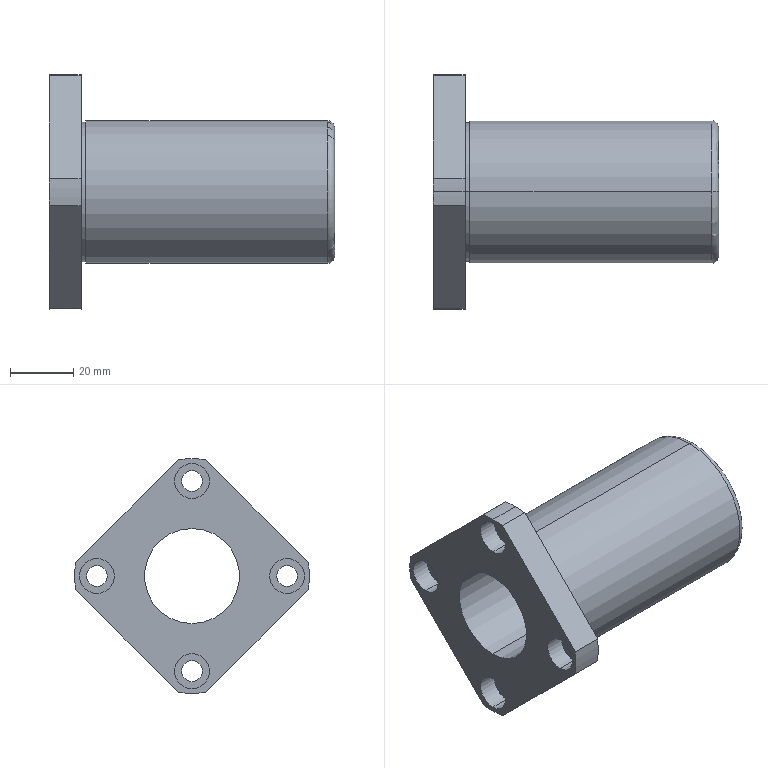Part | STEP file | 11-LHFSD3011 | 1 solid | 41 faces | box 90 x 74 x 74 mm | volume 93480 mm3 | cylinder 27 | plane 12 | torus 2 | commonest cylinder face diameters 6.6 x8 11 x8 74 x5 30 x2 44 x2 45 x2
STEP:
#1=CARTESIAN_POINT('',(10.,-30.,-3.3));
#2=VERTEX_POINT('',#1);
#3=CARTESIAN_POINT('',(10.,-30.,3.3));
#4=VERTEX_POINT('',#3);
#5=CARTESIAN_POINT('',(10.,-30.,0.));
#6=DIRECTION('',(-1.,0.,0.));
#7=DIRECTION('',(0.,0.,1.));
#8=AXIS2_PLACEMENT_3D('',#5,#6,#7);
#9=CIRCLE('',#8,3.3);
#10=EDGE_CURVE('',#2,#4,#9,.T.);
#11=ORIENTED_EDGE('',*,*,#10,.F.);
#12=CARTESIAN_POINT('',(6.1,-30.,-3.3));
#13=VERTEX_POINT('',#12);
#14=CARTESIAN_POINT('',(10.,-30.,-3.3));
#15=DIRECTION('',(-1.,0.,0.));
#16=VECTOR('',#15,1000.);
#17=LINE('',#14,#16);
#18=EDGE_CURVE('',#2,#13,#17,.T.);
#19=ORIENTED_EDGE('',*,*,#18,.T.);
#20=CARTESIAN_POINT('',(6.1,-30.,3.3));
#21=VERTEX_POINT('',#20);
#22=CARTESIAN_POINT('',(6.1,-30.,0.));
#23=DIRECTION('',(-1.,0.,0.));
#24=DIRECTION('',(0.,0.,1.));
#25=AXIS2_PLACEMENT_3D('',#22,#23,#24);
#26=CIRCLE('',#25,3.3);
#27=EDGE_CURVE('',#13,#21,#26,.T.);
#28=ORIENTED_EDGE('',*,*,#27,.T.);
#29=CARTESIAN_POINT('',(10.,-30.,3.3));
#30=DIRECTION('',(-1.,0.,0.));
#31=VECTOR('',#30,1000.);
#32=LINE('',#29,#31);
#33=EDGE_CURVE('',#4,#21,#32,.T.);
#34=ORIENTED_EDGE('',*,*,#33,.F.);
#35=EDGE_LOOP('',(#11,#19,#28,#34));
#36=FACE_OUTER_BOUND('',#35,.T.);
#37=CARTESIAN_POINT('',(10.,-30.,0.));
#38=DIRECTION('',(-1.,0.,0.));
#39=DIRECTION('',(0.,0.,1.));
#40=AXIS2_PLACEMENT_3D('',#37,#38,#39);
#41=CYLINDRICAL_SURFACE('',#40,3.3);
#42=ADVANCED_FACE('',(#36),#41,.F.);
#43=CARTESIAN_POINT('',(6.1,-30.,-5.5));
#44=VERTEX_POINT('',#43);
#45=CARTESIAN_POINT('',(6.1,-30.,5.5));
#46=VERTEX_POINT('',#45);
#47=CARTESIAN_POINT('',(6.1,-30.,0.));
#48=DIRECTION('',(-1.,0.,0.));
#49=DIRECTION('',(0.,0.,1.));
#50=AXIS2_PLACEMENT_3D('',#47,#48,#49);
#51=CIRCLE('',#50,5.5);
#52=EDGE_CURVE('',#44,#46,#51,.T.);
#53=ORIENTED_EDGE('',*,*,#52,.F.);
#54=CARTESIAN_POINT('',(0.,-30.,-5.5));
#55=VERTEX_POINT('',#54);
#56=CARTESIAN_POINT('',(10.,-30.,-5.5));
#57=DIRECTION('',(-1.,0.,0.));
#58=VECTOR('',#57,1000.);
#59=LINE('',#56,#58);
#60=EDGE_CURVE('',#44,#55,#59,.T.);
#61=ORIENTED_EDGE('',*,*,#60,.T.);
#62=CARTESIAN_POINT('',(0.,-30.,5.5));
#63=VERTEX_POINT('',#62);
#64=CARTESIAN_POINT('',(0.,-30.,0.));
#65=DIRECTION('',(-1.,0.,0.));
#66=DIRECTION('',(0.,0.,1.));
#67=AXIS2_PLACEMENT_3D('',#64,#65,#66);
#68=CIRCLE('',#67,5.5);
#69=EDGE_CURVE('',#55,#63,#68,.T.);
#70=ORIENTED_EDGE('',*,*,#69,.T.);
#71=CARTESIAN_POINT('',(10.,-30.,5.5));
#72=DIRECTION('',(-1.,0.,0.));
#73=VECTOR('',#72,1000.);
#74=LINE('',#71,#73);
#75=EDGE_CURVE('',#46,#63,#74,.T.);
#76=ORIENTED_EDGE('',*,*,#75,.F.);
#77=EDGE_LOOP('',(#53,#61,#70,#76));
#78=FACE_OUTER_BOUND('',#77,.T.);
#79=CARTESIAN_POINT('',(10.,-30.,0.));
#80=DIRECTION('',(-1.,0.,0.));
#81=DIRECTION('',(0.,0.,1.));
#82=AXIS2_PLACEMENT_3D('',#79,#80,#81);
#83=CYLINDRICAL_SURFACE('',#82,5.5);
#84=ADVANCED_FACE('',(#78),#83,.F.);
#85=CARTESIAN_POINT('',(10.,0.,26.7));
#86=VERTEX_POINT('',#85);
#87=CARTESIAN_POINT('',(10.,0.,33.3));
#88=VERTEX_POINT('',#87);
#89=CARTESIAN_POINT('',(10.,0.,30.));
#90=DIRECTION('',(-1.,0.,0.));
#91=DIRECTION('',(0.,0.,1.));
#92=AXIS2_PLACEMENT_3D('',#89,#90,#91);
#93=CIRCLE('',#92,3.3);
#94=EDGE_CURVE('',#86,#88,#93,.T.);
#95=ORIENTED_EDGE('',*,*,#94,.F.);
#96=CARTESIAN_POINT('',(6.1,0.,26.7));
#97=VERTEX_POINT('',#96);
#98=CARTESIAN_POINT('',(10.,0.,26.7));
#99=DIRECTION('',(-1.,0.,0.));
#100=VECTOR('',#99,1000.);
#101=LINE('',#98,#100);
#102=EDGE_CURVE('',#86,#97,#101,.T.);
#103=ORIENTED_EDGE('',*,*,#102,.T.);
#104=CARTESIAN_POINT('',(6.1,0.,33.3));
#105=VERTEX_POINT('',#104);
#106=CARTESIAN_POINT('',(6.1,0.,30.));
#107=DIRECTION('',(-1.,0.,0.));
#108=DIRECTION('',(0.,0.,1.));
#109=AXIS2_PLACEMENT_3D('',#106,#107,#108);
#110=CIRCLE('',#109,3.3);
#111=EDGE_CURVE('',#97,#105,#110,.T.);
#112=ORIENTED_EDGE('',*,*,#111,.T.);
#113=CARTESIAN_POINT('',(10.,0.,33.3));
#114=DIRECTION('',(-1.,0.,0.));
#115=VECTOR('',#114,1000.);
#116=LINE('',#113,#115);
#117=EDGE_CURVE('',#88,#105,#116,.T.);
#118=ORIENTED_EDGE('',*,*,#117,.F.);
#119=EDGE_LOOP('',(#95,#103,#112,#118));
#120=FACE_OUTER_BOUND('',#119,.T.);
#121=CARTESIAN_POINT('',(10.,0.,30.));
#122=DIRECTION('',(-1.,0.,0.));
#123=DIRECTION('',(0.,0.,1.));
#124=AXIS2_PLACEMENT_3D('',#121,#122,#123);
#125=CYLINDRICAL_SURFACE('',#124,3.3);
#126=ADVANCED_FACE('',(#120),#125,.F.);
#127=CARTESIAN_POINT('',(6.1,0.,24.5));
#128=VERTEX_POINT('',#127);
#129=CARTESIAN_POINT('',(6.1,0.,35.5));
#130=VERTEX_POINT('',#129);
#131=CARTESIAN_POINT('',(6.1,0.,30.));
#132=DIRECTION('',(-1.,0.,0.));
#133=DIRECTION('',(0.,0.,1.));
#134=AXIS2_PLACEMENT_3D('',#131,#132,#133);
#135=CIRCLE('',#134,5.5);
#136=EDGE_CURVE('',#128,#130,#135,.T.);
#137=ORIENTED_EDGE('',*,*,#136,.F.);
#138=CARTESIAN_POINT('',(0.,0.,24.5));
#139=VERTEX_POINT('',#138);
#140=CARTESIAN_POINT('',(10.,0.,24.5));
#141=DIRECTION('',(-1.,0.,0.));
#142=VECTOR('',#141,1000.);
#143=LINE('',#140,#142);
#144=EDGE_CURVE('',#128,#139,#143,.T.);
#145=ORIENTED_EDGE('',*,*,#144,.T.);
#146=CARTESIAN_POINT('',(0.,0.,35.5));
#147=VERTEX_POINT('',#146);
#148=CARTESIAN_POINT('',(0.,0.,30.));
#149=DIRECTION('',(-1.,0.,0.));
#150=DIRECTION('',(0.,0.,1.));
#151=AXIS2_PLACEMENT_3D('',#148,#149,#150);
#152=CIRCLE('',#151,5.5);
#153=EDGE_CURVE('',#139,#147,#152,.T.);
#154=ORIENTED_EDGE('',*,*,#153,.T.);
#155=CARTESIAN_POINT('',(10.,0.,35.5));
#156=DIRECTION('',(-1.,0.,0.));
#157=VECTOR('',#156,1000.);
#158=LINE('',#155,#157);
#159=EDGE_CURVE('',#130,#147,#158,.T.);
#160=ORIENTED_EDGE('',*,*,#159,.F.);
#161=EDGE_LOOP('',(#137,#145,#154,#160));
#162=FACE_OUTER_BOUND('',#161,.T.);
#163=CARTESIAN_POINT('',(10.,0.,30.));
#164=DIRECTION('',(-1.,0.,0.));
#165=DIRECTION('',(0.,0.,1.));
#166=AXIS2_PLACEMENT_3D('',#163,#164,#165);
#167=CYLINDRICAL_SURFACE('',#166,5.5);
#168=ADVANCED_FACE('',(#162),#167,.F.);
#169=CARTESIAN_POINT('',(10.,0.,-33.3));
#170=VERTEX_POINT('',#169);
#171=CARTESIAN_POINT('',(10.,0.,-26.7));
#172=VERTEX_POINT('',#171);
#173=CARTESIAN_POINT('',(10.,0.,-30.));
#174=DIRECTION('',(-1.,0.,0.));
#175=DIRECTION('',(0.,0.,1.));
#176=AXIS2_PLACEMENT_3D('',#173,#174,#175);
#177=CIRCLE('',#176,3.3);
#178=EDGE_CURVE('',#170,#172,#177,.T.);
#179=ORIENTED_EDGE('',*,*,#178,.F.);
#180=CARTESIAN_POINT('',(6.1,0.,-33.3));
#181=VERTEX_POINT('',#180);
#182=CARTESIAN_POINT('',(10.,0.,-33.3));
#183=DIRECTION('',(-1.,0.,0.));
#184=VECTOR('',#183,1000.);
#185=LINE('',#182,#184);
#186=EDGE_CURVE('',#170,#181,#185,.T.);
#187=ORIENTED_EDGE('',*,*,#186,.T.);
#188=CARTESIAN_POINT('',(6.1,0.,-26.7));
#189=VERTEX_POINT('',#188);
#190=CARTESIAN_POINT('',(6.1,0.,-30.));
#191=DIRECTION('',(-1.,0.,0.));
#192=DIRECTION('',(0.,0.,1.));
#193=AXIS2_PLACEMENT_3D('',#190,#191,#192);
#194=CIRCLE('',#193,3.3);
#195=EDGE_CURVE('',#181,#189,#194,.T.);
#196=ORIENTED_EDGE('',*,*,#195,.T.);
#197=CARTESIAN_POINT('',(10.,0.,-26.7));
#198=DIRECTION('',(-1.,0.,0.));
#199=VECTOR('',#198,1000.);
#200=LINE('',#197,#199);
#201=EDGE_CURVE('',#172,#189,#200,.T.);
#202=ORIENTED_EDGE('',*,*,#201,.F.);
#203=EDGE_LOOP('',(#179,#187,#196,#202));
#204=FACE_OUTER_BOUND('',#203,.T.);
#205=CARTESIAN_POINT('',(10.,0.,-30.));
#206=DIRECTION('',(-1.,0.,0.));
#207=DIRECTION('',(0.,0.,1.));
#208=AXIS2_PLACEMENT_3D('',#205,#206,#207);
#209=CYLINDRICAL_SURFACE('',#208,3.3);
#210=ADVANCED_FACE('',(#204),#209,.F.);
#211=CARTESIAN_POINT('',(6.1,0.,-35.5));
#212=VERTEX_POINT('',#211);
#213=CARTESIAN_POINT('',(6.1,0.,-24.5));
#214=VERTEX_POINT('',#213);
#215=CARTESIAN_POINT('',(6.1,0.,-30.));
#216=DIRECTION('',(-1.,0.,0.));
#217=DIRECTION('',(0.,0.,1.));
#218=AXIS2_PLACEMENT_3D('',#215,#216,#217);
#219=CIRCLE('',#218,5.5);
#220=EDGE_CURVE('',#212,#214,#219,.T.);
#221=ORIENTED_EDGE('',*,*,#220,.F.);
#222=CARTESIAN_POINT('',(0.,0.,-35.5));
#223=VERTEX_POINT('',#222);
#224=CARTESIAN_POINT('',(10.,0.,-35.5));
#225=DIRECTION('',(-1.,0.,0.));
#226=VECTOR('',#225,1000.);
#227=LINE('',#224,#226);
#228=EDGE_CURVE('',#212,#223,#227,.T.);
#229=ORIENTED_EDGE('',*,*,#228,.T.);
#230=CARTESIAN_POINT('',(0.,0.,-24.5));
#231=VERTEX_POINT('',#230);
#232=CARTESIAN_POINT('',(0.,0.,-30.));
#233=DIRECTION('',(-1.,0.,0.));
#234=DIRECTION('',(0.,0.,1.));
#235=AXIS2_PLACEMENT_3D('',#232,#233,#234);
#236=CIRCLE('',#235,5.5);
#237=EDGE_CURVE('',#223,#231,#236,.T.);
#238=ORIENTED_EDGE('',*,*,#237,.T.);
#239=CARTESIAN_POINT('',(10.,0.,-24.5));
#240=DIRECTION('',(-1.,0.,0.));
#241=VECTOR('',#240,1000.);
#242=LINE('',#239,#241);
#243=EDGE_CURVE('',#214,#231,#242,.T.);
#244=ORIENTED_EDGE('',*,*,#243,.F.);
#245=EDGE_LOOP('',(#221,#229,#238,#244));
#246=FACE_OUTER_BOUND('',#245,.T.);
#247=CARTESIAN_POINT('',(10.,0.,-30.));
#248=DIRECTION('',(-1.,0.,0.));
#249=DIRECTION('',(0.,0.,1.));
#250=AXIS2_PLACEMENT_3D('',#247,#248,#249);
#251=CYLINDRICAL_SURFACE('',#250,5.5);
#252=ADVANCED_FACE('',(#246),#251,.F.);
#253=CARTESIAN_POINT('',(10.,30.,-3.3));
#254=VERTEX_POINT('',#253);
#255=CARTESIAN_POINT('',(10.,30.,3.3));
#256=VERTEX_POINT('',#255);
#257=CARTESIAN_POINT('',(10.,30.,0.));
#258=DIRECTION('',(-1.,0.,0.));
#259=DIRECTION('',(0.,0.,1.));
#260=AXIS2_PLACEMENT_3D('',#257,#258,#259);
#261=CIRCLE('',#260,3.3);
#262=EDGE_CURVE('',#254,#256,#261,.T.);
#263=ORIENTED_EDGE('',*,*,#262,.F.);
#264=CARTESIAN_POINT('',(6.1,30.,-3.3));
#265=VERTEX_POINT('',#264);
#266=CARTESIAN_POINT('',(10.,30.,-3.3));
#267=DIRECTION('',(-1.,0.,0.));
#268=VECTOR('',#267,1000.);
#269=LINE('',#266,#268);
#270=EDGE_CURVE('',#254,#265,#269,.T.);
#271=ORIENTED_EDGE('',*,*,#270,.T.);
#272=CARTESIAN_POINT('',(6.1,30.,3.3));
#273=VERTEX_POINT('',#272);
#274=CARTESIAN_POINT('',(6.1,30.,0.));
#275=DIRECTION('',(-1.,0.,0.));
#276=DIRECTION('',(0.,0.,1.));
#277=AXIS2_PLACEMENT_3D('',#274,#275,#276);
#278=CIRCLE('',#277,3.3);
#279=EDGE_CURVE('',#265,#273,#278,.T.);
#280=ORIENTED_EDGE('',*,*,#279,.T.);
#281=CARTESIAN_POINT('',(10.,30.,3.3));
#282=DIRECTION('',(-1.,0.,0.));
#283=VECTOR('',#282,1000.);
#284=LINE('',#281,#283);
#285=EDGE_CURVE('',#256,#273,#284,.T.);
#286=ORIENTED_EDGE('',*,*,#285,.F.);
#287=EDGE_LOOP('',(#263,#271,#280,#286));
#288=FACE_OUTER_BOUND('',#287,.T.);
#289=CARTESIAN_POINT('',(10.,30.,0.));
#290=DIRECTION('',(-1.,0.,0.));
#291=DIRECTION('',(0.,0.,1.));
#292=AXIS2_PLACEMENT_3D('',#289,#290,#291);
#293=CYLINDRICAL_SURFACE('',#292,3.3);
#294=ADVANCED_FACE('',(#288),#293,.F.);
#295=CARTESIAN_POINT('',(6.1,30.,-5.5));
#296=VERTEX_POINT('',#295);
#297=CARTESIAN_POINT('',(6.1,30.,5.5));
#298=VERTEX_POINT('',#297);
#299=CARTESIAN_POINT('',(6.1,30.,0.));
#300=DIRECTION('',(-1.,0.,0.));
#301=DIRECTION('',(0.,0.,1.));
#302=AXIS2_PLACEMENT_3D('',#299,#300,#301);
#303=CIRCLE('',#302,5.5);
#304=EDGE_CURVE('',#296,#298,#303,.T.);
#305=ORIENTED_EDGE('',*,*,#304,.F.);
#306=CARTESIAN_POINT('',(0.,30.,-5.5));
#307=VERTEX_POINT('',#306);
#308=CARTESIAN_POINT('',(10.,30.,-5.5));
#309=DIRECTION('',(-1.,0.,0.));
#310=VECTOR('',#309,1000.);
#311=LINE('',#308,#310);
#312=EDGE_CURVE('',#296,#307,#311,.T.);
#313=ORIENTED_EDGE('',*,*,#312,.T.);
#314=CARTESIAN_POINT('',(0.,30.,5.5));
#315=VERTEX_POINT('',#314);
#316=CARTESIAN_POINT('',(0.,30.,0.));
#317=DIRECTION('',(-1.,0.,0.));
#318=DIRECTION('',(0.,0.,1.));
#319=AXIS2_PLACEMENT_3D('',#316,#317,#318);
#320=CIRCLE('',#319,5.5);
#321=EDGE_CURVE('',#307,#315,#320,.T.);
#322=ORIENTED_EDGE('',*,*,#321,.T.);
#323=CARTESIAN_POINT('',(10.,30.,5.5));
#324=DIRECTION('',(-1.,0.,0.));
#325=VECTOR('',#324,1000.);
#326=LINE('',#323,#325);
#327=EDGE_CURVE('',#298,#315,#326,.T.);
#328=ORIENTED_EDGE('',*,*,#327,.F.);
#329=EDGE_LOOP('',(#305,#313,#322,#328));
#330=FACE_OUTER_BOUND('',#329,.T.);
#331=CARTESIAN_POINT('',(10.,30.,0.));
#332=DIRECTION('',(-1.,0.,0.));
#333=DIRECTION('',(0.,0.,1.));
#334=AXIS2_PLACEMENT_3D('',#331,#332,#333);
#335=CYLINDRICAL_SURFACE('',#334,5.5);
#336=ADVANCED_FACE('',(#330),#335,.F.);
#337=CARTESIAN_POINT('',(11.5,0.,22.));
#338=VERTEX_POINT('',#337);
#339=CARTESIAN_POINT('',(11.5,0.,-22.));
#340=VERTEX_POINT('',#339);
#341=CARTESIAN_POINT('',(11.5,0.,0.));
#342=DIRECTION('',(-1.,0.,0.));
#343=DIRECTION('',(0.,0.,1.));
#344=AXIS2_PLACEMENT_3D('',#341,#342,#343);
#345=CIRCLE('',#344,22.);
#346=EDGE_CURVE('',#338,#340,#345,.T.);
#347=ORIENTED_EDGE('',*,*,#346,.T.);
#348=CARTESIAN_POINT('',(10.,0.,-22.));
#349=VERTEX_POINT('',#348);
#350=CARTESIAN_POINT('',(90.,0.,-22.));
#351=DIRECTION('',(-1.,0.,0.));
#352=VECTOR('',#351,1000.);
#353=LINE('',#350,#352);
#354=EDGE_CURVE('',#340,#349,#353,.T.);
#355=ORIENTED_EDGE('',*,*,#354,.T.);
#356=CARTESIAN_POINT('',(10.,0.,22.));
#357=VERTEX_POINT('',#356);
#358=CARTESIAN_POINT('',(10.,0.,0.));
#359=DIRECTION('',(-1.,0.,0.));
#360=DIRECTION('',(0.,0.,1.));
#361=AXIS2_PLACEMENT_3D('',#358,#359,#360);
#362=CIRCLE('',#361,22.);
#363=EDGE_CURVE('',#357,#349,#362,.T.);
#364=ORIENTED_EDGE('',*,*,#363,.F.);
#365=CARTESIAN_POINT('',(90.,0.,22.));
#366=DIRECTION('',(-1.,0.,0.));
#367=VECTOR('',#366,1000.);
#368=LINE('',#365,#367);
#369=EDGE_CURVE('',#338,#357,#368,.T.);
#370=ORIENTED_EDGE('',*,*,#369,.F.);
#371=EDGE_LOOP('',(#347,#355,#364,#370));
#372=FACE_OUTER_BOUND('',#371,.T.);
#373=CARTESIAN_POINT('',(90.,0.,0.));
#374=DIRECTION('',(-1.,0.,0.));
#375=DIRECTION('',(0.,0.,1.));
#376=AXIS2_PLACEMENT_3D('',#373,#374,#375);
#377=CYLINDRICAL_SURFACE('',#376,22.);
#378=ADVANCED_FACE('',(#372),#377,.T.);
#379=CARTESIAN_POINT('',(87.75,0.,22.5));
#380=VERTEX_POINT('',#379);
#381=CARTESIAN_POINT('',(87.75,0.,-22.5));
#382=VERTEX_POINT('',#381);
#383=CARTESIAN_POINT('',(87.75,0.,0.));
#384=DIRECTION('',(-1.,0.,0.));
#385=DIRECTION('',(0.,0.,1.));
#386=AXIS2_PLACEMENT_3D('',#383,#384,#385);
#387=CIRCLE('',#386,22.5);
#388=EDGE_CURVE('',#380,#382,#387,.T.);
#389=ORIENTED_EDGE('',*,*,#388,.T.);
#390=CARTESIAN_POINT('',(11.5,0.,-22.5));
#391=VERTEX_POINT('',#390);
#392=CARTESIAN_POINT('',(90.,0.,-22.5));
#393=DIRECTION('',(-1.,0.,0.));
#394=VECTOR('',#393,1000.);
#395=LINE('',#392,#394);
#396=EDGE_CURVE('',#382,#391,#395,.T.);
#397=ORIENTED_EDGE('',*,*,#396,.T.);
#398=CARTESIAN_POINT('',(11.5,0.,22.5));
#399=VERTEX_POINT('',#398);
#400=CARTESIAN_POINT('',(11.5,0.,0.));
#401=DIRECTION('',(-1.,0.,0.));
#402=DIRECTION('',(0.,0.,1.));
#403=AXIS2_PLACEMENT_3D('',#400,#401,#402);
#404=CIRCLE('',#403,22.5);
#405=EDGE_CURVE('',#399,#391,#404,.T.);
#406=ORIENTED_EDGE('',*,*,#405,.F.);
#407=CARTESIAN_POINT('',(90.,0.,22.5));
#408=DIRECTION('',(-1.,0.,0.));
#409=VECTOR('',#408,1000.);
#410=LINE('',#407,#409);
#411=EDGE_CURVE('',#380,#399,#410,.T.);
#412=ORIENTED_EDGE('',*,*,#411,.F.);
#413=EDGE_LOOP('',(#389,#397,#406,#412));
#414=FACE_OUTER_BOUND('',#413,.T.);
#415=CARTESIAN_POINT('',(90.,0.,0.));
#416=DIRECTION('',(-1.,0.,0.));
#417=DIRECTION('',(0.,0.,1.));
#418=AXIS2_PLACEMENT_3D('',#415,#416,#417);
#419=CYLINDRICAL_SURFACE('',#418,22.5);
#420=ADVANCED_FACE('',(#414),#419,.T.);
#421=CARTESIAN_POINT('',(90.,0.,20.25));
#422=VERTEX_POINT('',#421);
#423=CARTESIAN_POINT('',(90.,0.,-20.25));
#424=VERTEX_POINT('',#423);
#425=CARTESIAN_POINT('',(90.,0.,0.));
#426=DIRECTION('',(-1.,0.,0.));
#427=DIRECTION('',(0.,0.,1.));
#428=AXIS2_PLACEMENT_3D('',#425,#426,#427);
#429=CIRCLE('',#428,20.25);
#430=EDGE_CURVE('',#422,#424,#429,.T.);
#431=ORIENTED_EDGE('',*,*,#430,.T.);
#432=CARTESIAN_POINT('',(87.75,0.,-20.25));
#433=DIRECTION('',(0.,1.,0.));
#434=DIRECTION('',(0.,0.,1.));
#435=AXIS2_PLACEMENT_3D('',#432,#433,#434);
#436=CIRCLE('',#435,2.25);
#437=EDGE_CURVE('',#424,#382,#436,.T.);
#438=ORIENTED_EDGE('',*,*,#437,.T.);
#439=ORIENTED_EDGE('',*,*,#388,.F.);
#440=CARTESIAN_POINT('',(87.75,0.,20.25));
#441=DIRECTION('',(0.,-1.,0.));
#442=DIRECTION('',(0.,0.,-1.));
#443=AXIS2_PLACEMENT_3D('',#440,#441,#442);
#444=CIRCLE('',#443,2.25);
#445=EDGE_CURVE('',#422,#380,#444,.T.);
#446=ORIENTED_EDGE('',*,*,#445,.F.);
#447=EDGE_LOOP('',(#431,#438,#439,#446));
#448=FACE_OUTER_BOUND('',#447,.T.);
#449=CARTESIAN_POINT('',(87.75,0.,0.));
#450=DIRECTION('',(-1.,0.,0.));
#451=DIRECTION('',(0.,0.,1.));
#452=AXIS2_PLACEMENT_3D('',#449,#450,#451);
#453=TOROIDAL_SURFACE('',#452,20.25,2.25);
#454=ADVANCED_FACE('',(#448),#453,.T.);
#455=CARTESIAN_POINT('',(90.,0.,-15.));
#456=VERTEX_POINT('',#455);
#457=CARTESIAN_POINT('',(90.,0.,15.));
#458=VERTEX_POINT('',#457);
#459=CARTESIAN_POINT('',(90.,0.,0.));
#460=DIRECTION('',(-1.,0.,0.));
#461=DIRECTION('',(0.,0.,1.));
#462=AXIS2_PLACEMENT_3D('',#459,#460,#461);
#463=CIRCLE('',#462,15.);
#464=EDGE_CURVE('',#456,#458,#463,.T.);
#465=ORIENTED_EDGE('',*,*,#464,.F.);
#466=CARTESIAN_POINT('',(0.,0.,-15.));
#467=VERTEX_POINT('',#466);
#468=CARTESIAN_POINT('',(90.,0.,-15.));
#469=DIRECTION('',(-1.,0.,0.));
#470=VECTOR('',#469,1000.);
#471=LINE('',#468,#470);
#472=EDGE_CURVE('',#456,#467,#471,.T.);
#473=ORIENTED_EDGE('',*,*,#472,.T.);
#474=CARTESIAN_POINT('',(0.,0.,15.));
#475=VERTEX_POINT('',#474);
#476=CARTESIAN_POINT('',(0.,0.,0.));
#477=DIRECTION('',(-1.,0.,0.));
#478=DIRECTION('',(0.,0.,1.));
#479=AXIS2_PLACEMENT_3D('',#476,#477,#478);
#480=CIRCLE('',#479,15.);
#481=EDGE_CURVE('',#467,#475,#480,.T.);
#482=ORIENTED_EDGE('',*,*,#481,.T.);
#483=CARTESIAN_POINT('',(90.,0.,15.));
#484=DIRECTION('',(-1.,0.,0.));
#485=VECTOR('',#484,1000.);
#486=LINE('',#483,#485);
#487=EDGE_CURVE('',#458,#475,#486,.T.);
#488=ORIENTED_EDGE('',*,*,#487,.F.);
#489=EDGE_LOOP('',(#465,#473,#482,#488));
#490=FACE_OUTER_BOUND('',#489,.T.);
#491=CARTESIAN_POINT('',(90.,0.,0.));
#492=DIRECTION('',(-1.,0.,0.));
#493=DIRECTION('',(0.,0.,1.));
#494=AXIS2_PLACEMENT_3D('',#491,#492,#493);
#495=CYLINDRICAL_SURFACE('',#494,15.);
#496=ADVANCED_FACE('',(#490),#495,.F.);
#497=CARTESIAN_POINT('',(10.,-4.258,36.754));
#498=VERTEX_POINT('',#497);
#499=CARTESIAN_POINT('',(10.,0.,37.));
#500=VERTEX_POINT('',#499);
#501=CARTESIAN_POINT('',(10.,0.,0.));
#502=DIRECTION('',(-1.,0.,0.));
#503=DIRECTION('',(0.,0.,1.));
#504=AXIS2_PLACEMENT_3D('',#501,#502,#503);
#505=CIRCLE('',#504,37.);
#506=EDGE_CURVE('',#498,#500,#505,.T.);
#507=ORIENTED_EDGE('',*,*,#506,.T.);
#508=CARTESIAN_POINT('',(0.,0.,37.));
#509=VERTEX_POINT('',#508);
#510=CARTESIAN_POINT('',(90.,0.,37.));
#511=DIRECTION('',(-1.,0.,0.));
#512=VECTOR('',#511,1000.);
#513=LINE('',#510,#512);
#514=EDGE_CURVE('',#500,#509,#513,.T.);
#515=ORIENTED_EDGE('',*,*,#514,.T.);
#516=CARTESIAN_POINT('',(0.,-4.258,36.754));
#517=VERTEX_POINT('',#516);
#518=CARTESIAN_POINT('',(0.,0.,0.));
#519=DIRECTION('',(-1.,0.,0.));
#520=DIRECTION('',(0.,0.,1.));
#521=AXIS2_PLACEMENT_3D('',#518,#519,#520);
#522=CIRCLE('',#521,37.);
#523=EDGE_CURVE('',#517,#509,#522,.T.);
#524=ORIENTED_EDGE('',*,*,#523,.F.);
#525=CARTESIAN_POINT('',(90.,-4.258,36.754));
#526=DIRECTION('',(1.,0.,0.));
#527=VECTOR('',#526,1000.);
#528=LINE('',#525,#527);
#529=EDGE_CURVE('',#517,#498,#528,.T.);
#530=ORIENTED_EDGE('',*,*,#529,.T.);
#531=EDGE_LOOP('',(#507,#515,#524,#530));
#532=FACE_OUTER_BOUND('',#531,.T.);
#533=CARTESIAN_POINT('',(90.,0.,0.));
#534=DIRECTION('',(-1.,0.,0.));
#535=DIRECTION('',(0.,0.,1.));
#536=AXIS2_PLACEMENT_3D('',#533,#534,#535);
#537=CYLINDRICAL_SURFACE('',#536,37.);
#538=ADVANCED_FACE('',(#532),#537,.T.);
#539=ORIENTED_EDGE('',*,*,#514,.F.);
#540=CARTESIAN_POINT('',(10.,4.258,36.754));
#541=VERTEX_POINT('',#540);
#542=CARTESIAN_POINT('',(10.,0.,0.));
#543=DIRECTION('',(-1.,0.,0.));
#544=DIRECTION('',(0.,0.,1.));
#545=AXIS2_PLACEMENT_3D('',#542,#543,#544);
#546=CIRCLE('',#545,37.);
#547=EDGE_CURVE('',#500,#541,#546,.T.);
#548=ORIENTED_EDGE('',*,*,#547,.T.);
#549=CARTESIAN_POINT('',(0.,4.258,36.754));
#550=VERTEX_POINT('',#549);
#551=CARTESIAN_POINT('',(90.,4.258,36.754));
#552=DIRECTION('',(-1.,0.,0.));
#553=VECTOR('',#552,1000.);
#554=LINE('',#551,#553);
#555=EDGE_CURVE('',#541,#550,#554,.T.);
#556=ORIENTED_EDGE('',*,*,#555,.T.);
#557=CARTESIAN_POINT('',(0.,0.,0.));
#558=DIRECTION('',(-1.,0.,0.));
#559=DIRECTION('',(0.,0.,1.));
#560=AXIS2_PLACEMENT_3D('',#557,#558,#559);
#561=CIRCLE('',#560,37.);
#562=EDGE_CURVE('',#509,#550,#561,.T.);
#563=ORIENTED_EDGE('',*,*,#562,.F.);
#564=EDGE_LOOP('',(#539,#548,#556,#563));
#565=FACE_OUTER_BOUND('',#564,.T.);
#566=CARTESIAN_POINT('',(90.,0.,0.));
#567=DIRECTION('',(-1.,0.,0.));
#568=DIRECTION('',(0.,0.,1.));
#569=AXIS2_PLACEMENT_3D('',#566,#567,#568);
#570=CYLINDRICAL_SURFACE('',#569,37.);
#571=ADVANCED_FACE('',(#565),#570,.T.);
#572=CARTESIAN_POINT('',(10.,-36.754,-4.258));
#573=VERTEX_POINT('',#572);
#574=CARTESIAN_POINT('',(10.,-36.754,4.258));
#575=VERTEX_POINT('',#574);
#576=CARTESIAN_POINT('',(10.,0.,0.));
#577=DIRECTION('',(-1.,0.,0.));
#578=DIRECTION('',(0.,0.,1.));
#579=AXIS2_PLACEMENT_3D('',#576,#577,#578);
#580=CIRCLE('',#579,37.);
#581=EDGE_CURVE('',#573,#575,#580,.T.);
#582=ORIENTED_EDGE('',*,*,#581,.T.);
#583=CARTESIAN_POINT('',(0.,-36.754,4.258));
#584=VERTEX_POINT('',#583);
#585=CARTESIAN_POINT('',(90.,-36.754,4.258));
#586=DIRECTION('',(-1.,0.,0.));
#587=VECTOR('',#586,1000.);
#588=LINE('',#585,#587);
#589=EDGE_CURVE('',#575,#584,#588,.T.);
#590=ORIENTED_EDGE('',*,*,#589,.T.);
#591=CARTESIAN_POINT('',(0.,-36.754,-4.258));
#592=VERTEX_POINT('',#591);
#593=CARTESIAN_POINT('',(0.,0.,0.));
#594=DIRECTION('',(-1.,0.,0.));
#595=DIRECTION('',(0.,0.,1.));
#596=AXIS2_PLACEMENT_3D('',#593,#594,#595);
#597=CIRCLE('',#596,37.);
#598=EDGE_CURVE('',#592,#584,#597,.T.);
#599=ORIENTED_EDGE('',*,*,#598,.F.);
#600=CARTESIAN_POINT('',(90.,-36.754,-4.258));
#601=DIRECTION('',(1.,0.,0.));
#602=VECTOR('',#601,1000.);
#603=LINE('',#600,#602);
#604=EDGE_CURVE('',#592,#573,#603,.T.);
#605=ORIENTED_EDGE('',*,*,#604,.T.);
#606=EDGE_LOOP('',(#582,#590,#599,#605));
#607=FACE_OUTER_BOUND('',#606,.T.);
#608=CARTESIAN_POINT('',(90.,0.,0.));
#609=DIRECTION('',(-1.,0.,0.));
#610=DIRECTION('',(0.,0.,1.));
#611=AXIS2_PLACEMENT_3D('',#608,#609,#610);
#612=CYLINDRICAL_SURFACE('',#611,37.);
#613=ADVANCED_FACE('',(#607),#612,.T.);
#614=CARTESIAN_POINT('',(10.,4.258,-36.754));
#615=VERTEX_POINT('',#614);
#616=CARTESIAN_POINT('',(10.,-4.258,-36.754));
#617=VERTEX_POINT('',#616);
#618=CARTESIAN_POINT('',(10.,0.,0.));
#619=DIRECTION('',(-1.,0.,0.));
#620=DIRECTION('',(0.,0.,1.));
#621=AXIS2_PLACEMENT_3D('',#618,#619,#620);
#622=CIRCLE('',#621,37.);
#623=EDGE_CURVE('',#615,#617,#622,.T.);
#624=ORIENTED_EDGE('',*,*,#623,.T.);
#625=CARTESIAN_POINT('',(0.,-4.258,-36.754));
#626=VERTEX_POINT('',#625);
#627=CARTESIAN_POINT('',(90.,-4.258,-36.754));
#628=DIRECTION('',(-1.,0.,0.));
#629=VECTOR('',#628,1000.);
#630=LINE('',#627,#629);
#631=EDGE_CURVE('',#617,#626,#630,.T.);
#632=ORIENTED_EDGE('',*,*,#631,.T.);
#633=CARTESIAN_POINT('',(0.,4.258,-36.754));
#634=VERTEX_POINT('',#633);
#635=CARTESIAN_POINT('',(0.,0.,0.));
#636=DIRECTION('',(-1.,0.,0.));
#637=DIRECTION('',(0.,0.,1.));
#638=AXIS2_PLACEMENT_3D('',#635,#636,#637);
#639=CIRCLE('',#638,37.);
#640=EDGE_CURVE('',#634,#626,#639,.T.);
#641=ORIENTED_EDGE('',*,*,#640,.F.);
#642=CARTESIAN_POINT('',(90.,4.258,-36.754));
#643=DIRECTION('',(1.,0.,0.));
#644=VECTOR('',#643,1000.);
#645=LINE('',#642,#644);
#646=EDGE_CURVE('',#634,#615,#645,.T.);
#647=ORIENTED_EDGE('',*,*,#646,.T.);
#648=EDGE_LOOP('',(#624,#632,#641,#647));
#649=FACE_OUTER_BOUND('',#648,.T.);
#650=CARTESIAN_POINT('',(90.,0.,0.));
#651=DIRECTION('',(-1.,0.,0.));
#652=DIRECTION('',(0.,0.,1.));
#653=AXIS2_PLACEMENT_3D('',#650,#651,#652);
#654=CYLINDRICAL_SURFACE('',#653,37.);
#655=ADVANCED_FACE('',(#649),#654,.T.);
#656=CARTESIAN_POINT('',(0.,-30.,0.));
#657=DIRECTION('',(-1.,0.,0.));
#658=DIRECTION('',(0.,0.,1.));
#659=AXIS2_PLACEMENT_3D('',#656,#657,#658);
#660=CIRCLE('',#659,5.5);
#661=EDGE_CURVE('',#63,#55,#660,.T.);
#662=ORIENTED_EDGE('',*,*,#661,.F.);
#663=ORIENTED_EDGE('',*,*,#69,.F.);
#664=EDGE_LOOP('',(#662,#663));
#665=FACE_BOUND('',#664,.T.);
#666=CARTESIAN_POINT('',(0.,0.,30.));
#667=DIRECTION('',(-1.,0.,0.));
#668=DIRECTION('',(0.,0.,1.));
#669=AXIS2_PLACEMENT_3D('',#666,#667,#668);
#670=CIRCLE('',#669,5.5);
#671=EDGE_CURVE('',#147,#139,#670,.T.);
#672=ORIENTED_EDGE('',*,*,#671,.F.);
#673=ORIENTED_EDGE('',*,*,#153,.F.);
#674=EDGE_LOOP('',(#672,#673));
#675=FACE_BOUND('',#674,.T.);
#676=CARTESIAN_POINT('',(0.,0.,-30.));
#677=DIRECTION('',(-1.,0.,0.));
#678=DIRECTION('',(0.,0.,1.));
#679=AXIS2_PLACEMENT_3D('',#676,#677,#678);
#680=CIRCLE('',#679,5.5);
#681=EDGE_CURVE('',#231,#223,#680,.T.);
#682=ORIENTED_EDGE('',*,*,#681,.F.);
#683=ORIENTED_EDGE('',*,*,#237,.F.);
#684=EDGE_LOOP('',(#682,#683));
#685=FACE_BOUND('',#684,.T.);
#686=CARTESIAN_POINT('',(0.,30.,0.));
#687=DIRECTION('',(-1.,0.,0.));
#688=DIRECTION('',(0.,0.,1.));
#689=AXIS2_PLACEMENT_3D('',#686,#687,#688);
#690=CIRCLE('',#689,5.5);
#691=EDGE_CURVE('',#315,#307,#690,.T.);
#692=ORIENTED_EDGE('',*,*,#691,.F.);
#693=ORIENTED_EDGE('',*,*,#321,.F.);
#694=EDGE_LOOP('',(#692,#693));
#695=FACE_BOUND('',#694,.T.);
#696=CARTESIAN_POINT('',(0.,0.,0.));
#697=DIRECTION('',(-1.,0.,0.));
#698=DIRECTION('',(0.,0.,1.));
#699=AXIS2_PLACEMENT_3D('',#696,#697,#698);
#700=CIRCLE('',#699,15.);
#701=EDGE_CURVE('',#475,#467,#700,.T.);
#702=ORIENTED_EDGE('',*,*,#701,.F.);
#703=ORIENTED_EDGE('',*,*,#481,.F.);
#704=EDGE_LOOP('',(#702,#703));
#705=FACE_BOUND('',#704,.T.);
#706=ORIENTED_EDGE('',*,*,#598,.T.);
#707=CARTESIAN_POINT('',(0.,-4.012,37.));
#708=DIRECTION('',(0.,-0.7071,-0.7071));
#709=VECTOR('',#708,1000.);
#710=LINE('',#707,#709);
#711=EDGE_CURVE('',#517,#584,#710,.T.);
#712=ORIENTED_EDGE('',*,*,#711,.F.);
#713=ORIENTED_EDGE('',*,*,#523,.T.);
#714=ORIENTED_EDGE('',*,*,#562,.T.);
#715=CARTESIAN_POINT('',(0.,36.754,4.258));
#716=VERTEX_POINT('',#715);
#717=CARTESIAN_POINT('',(0.,37.,4.012));
#718=DIRECTION('',(0.,-0.7071,0.7071));
#719=VECTOR('',#718,1000.);
#720=LINE('',#717,#719);
#721=EDGE_CURVE('',#716,#550,#720,.T.);
#722=ORIENTED_EDGE('',*,*,#721,.F.);
#723=CARTESIAN_POINT('',(0.,36.754,-4.258));
#724=VERTEX_POINT('',#723);
#725=CARTESIAN_POINT('',(0.,0.,0.));
#726=DIRECTION('',(-1.,0.,0.));
#727=DIRECTION('',(0.,0.,1.));
#728=AXIS2_PLACEMENT_3D('',#725,#726,#727);
#729=CIRCLE('',#728,37.);
#730=EDGE_CURVE('',#716,#724,#729,.T.);
#731=ORIENTED_EDGE('',*,*,#730,.T.);
#732=CARTESIAN_POINT('',(0.,4.012,-37.));
#733=DIRECTION('',(0.,0.7071,0.7071));
#734=VECTOR('',#733,1000.);
#735=LINE('',#732,#734);
#736=EDGE_CURVE('',#634,#724,#735,.T.);
#737=ORIENTED_EDGE('',*,*,#736,.F.);
#738=ORIENTED_EDGE('',*,*,#640,.T.);
#739=CARTESIAN_POINT('',(0.,-37.,-4.012));
#740=DIRECTION('',(0.,0.7071,-0.7071));
#741=VECTOR('',#740,1000.);
#742=LINE('',#739,#741);
#743=EDGE_CURVE('',#592,#626,#742,.T.);
#744=ORIENTED_EDGE('',*,*,#743,.F.);
#745=EDGE_LOOP('',(#706,#712,#713,#714,#722,#731,#737,#738,#744));
#746=FACE_OUTER_BOUND('',#745,.T.);
#747=CARTESIAN_POINT('',(0.,37.,0.));
#748=DIRECTION('',(1.,0.,0.));
#749=DIRECTION('',(0.,0.,-1.));
#750=AXIS2_PLACEMENT_3D('',#747,#748,#749);
#751=PLANE('',#750);
#752=ADVANCED_FACE('',(#665,#675,#685,#695,#705,#746),#751,.F.);
#753=ORIENTED_EDGE('',*,*,#472,.F.);
#754=CARTESIAN_POINT('',(90.,0.,0.));
#755=DIRECTION('',(-1.,0.,0.));
#756=DIRECTION('',(0.,0.,1.));
#757=AXIS2_PLACEMENT_3D('',#754,#755,#756);
#758=CIRCLE('',#757,15.);
#759=EDGE_CURVE('',#458,#456,#758,.T.);
#760=ORIENTED_EDGE('',*,*,#759,.F.);
#761=ORIENTED_EDGE('',*,*,#487,.T.);
#762=ORIENTED_EDGE('',*,*,#701,.T.);
#763=EDGE_LOOP('',(#753,#760,#761,#762));
#764=FACE_OUTER_BOUND('',#763,.T.);
#765=CARTESIAN_POINT('',(90.,0.,0.));
#766=DIRECTION('',(-1.,0.,0.));
#767=DIRECTION('',(0.,0.,1.));
#768=AXIS2_PLACEMENT_3D('',#765,#766,#767);
#769=CYLINDRICAL_SURFACE('',#768,15.);
#770=ADVANCED_FACE('',(#764),#769,.F.);
#771=ORIENTED_EDGE('',*,*,#430,.F.);
#772=CARTESIAN_POINT('',(90.,0.,0.));
#773=DIRECTION('',(-1.,0.,0.));
#774=DIRECTION('',(0.,0.,1.));
#775=AXIS2_PLACEMENT_3D('',#772,#773,#774);
#776=CIRCLE('',#775,20.25);
#777=EDGE_CURVE('',#424,#422,#776,.T.);
#778=ORIENTED_EDGE('',*,*,#777,.F.);
#779=EDGE_LOOP('',(#771,#778));
#780=FACE_OUTER_BOUND('',#779,.T.);
#781=ORIENTED_EDGE('',*,*,#759,.T.);
#782=ORIENTED_EDGE('',*,*,#464,.T.);
#783=EDGE_LOOP('',(#781,#782));
#784=FACE_BOUND('',#783,.T.);
#785=CARTESIAN_POINT('',(90.,15.,0.));
#786=DIRECTION('',(-1.,0.,0.));
#787=DIRECTION('',(0.,0.,1.));
#788=AXIS2_PLACEMENT_3D('',#785,#786,#787);
#789=PLANE('',#788);
#790=ADVANCED_FACE('',(#780,#784),#789,.F.);
#791=ORIENTED_EDGE('',*,*,#437,.F.);
#792=ORIENTED_EDGE('',*,*,#777,.T.);
#793=ORIENTED_EDGE('',*,*,#445,.T.);
#794=CARTESIAN_POINT('',(87.75,0.,0.));
#795=DIRECTION('',(-1.,0.,0.));
#796=DIRECTION('',(0.,0.,1.));
#797=AXIS2_PLACEMENT_3D('',#794,#795,#796);
#798=CIRCLE('',#797,22.5);
#799=EDGE_CURVE('',#382,#380,#798,.T.);
#800=ORIENTED_EDGE('',*,*,#799,.F.);
#801=EDGE_LOOP('',(#791,#792,#793,#800));
#802=FACE_OUTER_BOUND('',#801,.T.);
#803=CARTESIAN_POINT('',(87.75,0.,0.));
#804=DIRECTION('',(-1.,0.,0.));
#805=DIRECTION('',(0.,0.,1.));
#806=AXIS2_PLACEMENT_3D('',#803,#804,#805);
#807=TOROIDAL_SURFACE('',#806,20.25,2.25);
#808=ADVANCED_FACE('',(#802),#807,.T.);
#809=ORIENTED_EDGE('',*,*,#396,.F.);
#810=ORIENTED_EDGE('',*,*,#799,.T.);
#811=ORIENTED_EDGE('',*,*,#411,.T.);
#812=CARTESIAN_POINT('',(11.5,0.,0.));
#813=DIRECTION('',(-1.,0.,0.));
#814=DIRECTION('',(0.,0.,1.));
#815=AXIS2_PLACEMENT_3D('',#812,#813,#814);
#816=CIRCLE('',#815,22.5);
#817=EDGE_CURVE('',#391,#399,#816,.T.);
#818=ORIENTED_EDGE('',*,*,#817,.F.);
#819=EDGE_LOOP('',(#809,#810,#811,#818));
#820=FACE_OUTER_BOUND('',#819,.T.);
#821=CARTESIAN_POINT('',(90.,0.,0.));
#822=DIRECTION('',(-1.,0.,0.));
#823=DIRECTION('',(0.,0.,1.));
#824=AXIS2_PLACEMENT_3D('',#821,#822,#823);
#825=CYLINDRICAL_SURFACE('',#824,22.5);
#826=ADVANCED_FACE('',(#820),#825,.T.);
#827=ORIENTED_EDGE('',*,*,#346,.F.);
#828=CARTESIAN_POINT('',(11.5,0.,0.));
#829=DIRECTION('',(-1.,0.,0.));
#830=DIRECTION('',(0.,0.,1.));
#831=AXIS2_PLACEMENT_3D('',#828,#829,#830);
#832=CIRCLE('',#831,22.);
#833=EDGE_CURVE('',#340,#338,#832,.T.);
#834=ORIENTED_EDGE('',*,*,#833,.F.);
#835=EDGE_LOOP('',(#827,#834));
#836=FACE_BOUND('',#835,.T.);
#837=ORIENTED_EDGE('',*,*,#405,.T.);
#838=ORIENTED_EDGE('',*,*,#817,.T.);
#839=EDGE_LOOP('',(#837,#838));
#840=FACE_OUTER_BOUND('',#839,.T.);
#841=CARTESIAN_POINT('',(11.5,22.5,0.));
#842=DIRECTION('',(1.,0.,0.));
#843=DIRECTION('',(0.,0.,-1.));
#844=AXIS2_PLACEMENT_3D('',#841,#842,#843);
#845=PLANE('',#844);
#846=ADVANCED_FACE('',(#836,#840),#845,.F.);
#847=ORIENTED_EDGE('',*,*,#354,.F.);
#848=ORIENTED_EDGE('',*,*,#833,.T.);
#849=ORIENTED_EDGE('',*,*,#369,.T.);
#850=CARTESIAN_POINT('',(10.,0.,0.));
#851=DIRECTION('',(-1.,0.,0.));
#852=DIRECTION('',(0.,0.,1.));
#853=AXIS2_PLACEMENT_3D('',#850,#851,#852);
#854=CIRCLE('',#853,22.);
#855=EDGE_CURVE('',#349,#357,#854,.T.);
#856=ORIENTED_EDGE('',*,*,#855,.F.);
#857=EDGE_LOOP('',(#847,#848,#849,#856));
#858=FACE_OUTER_BOUND('',#857,.T.);
#859=CARTESIAN_POINT('',(90.,0.,0.));
#860=DIRECTION('',(-1.,0.,0.));
#861=DIRECTION('',(0.,0.,1.));
#862=AXIS2_PLACEMENT_3D('',#859,#860,#861);
#863=CYLINDRICAL_SURFACE('',#862,22.);
#864=ADVANCED_FACE('',(#858),#863,.T.);
#865=CARTESIAN_POINT('',(10.,-30.,0.));
#866=DIRECTION('',(-1.,0.,0.));
#867=DIRECTION('',(0.,0.,1.));
#868=AXIS2_PLACEMENT_3D('',#865,#866,#867);
#869=CIRCLE('',#868,3.3);
#870=EDGE_CURVE('',#4,#2,#869,.T.);
#871=ORIENTED_EDGE('',*,*,#870,.T.);
#872=ORIENTED_EDGE('',*,*,#10,.T.);
#873=EDGE_LOOP('',(#871,#872));
#874=FACE_BOUND('',#873,.T.);
#875=CARTESIAN_POINT('',(10.,0.,30.));
#876=DIRECTION('',(-1.,0.,0.));
#877=DIRECTION('',(0.,0.,1.));
#878=AXIS2_PLACEMENT_3D('',#875,#876,#877);
#879=CIRCLE('',#878,3.3);
#880=EDGE_CURVE('',#88,#86,#879,.T.);
#881=ORIENTED_EDGE('',*,*,#880,.T.);
#882=ORIENTED_EDGE('',*,*,#94,.T.);
#883=EDGE_LOOP('',(#881,#882));
#884=FACE_BOUND('',#883,.T.);
#885=CARTESIAN_POINT('',(10.,0.,-30.));
#886=DIRECTION('',(-1.,0.,0.));
#887=DIRECTION('',(0.,0.,1.));
#888=AXIS2_PLACEMENT_3D('',#885,#886,#887);
#889=CIRCLE('',#888,3.3);
#890=EDGE_CURVE('',#172,#170,#889,.T.);
#891=ORIENTED_EDGE('',*,*,#890,.T.);
#892=ORIENTED_EDGE('',*,*,#178,.T.);
#893=EDGE_LOOP('',(#891,#892));
#894=FACE_BOUND('',#893,.T.);
#895=CARTESIAN_POINT('',(10.,30.,0.));
#896=DIRECTION('',(-1.,0.,0.));
#897=DIRECTION('',(0.,0.,1.));
#898=AXIS2_PLACEMENT_3D('',#895,#896,#897);
#899=CIRCLE('',#898,3.3);
#900=EDGE_CURVE('',#256,#254,#899,.T.);
#901=ORIENTED_EDGE('',*,*,#900,.T.);
#902=ORIENTED_EDGE('',*,*,#262,.T.);
#903=EDGE_LOOP('',(#901,#902));
#904=FACE_BOUND('',#903,.T.);
#905=ORIENTED_EDGE('',*,*,#506,.F.);
#906=CARTESIAN_POINT('',(10.,-4.012,37.));
#907=DIRECTION('',(0.,-0.7071,-0.7071));
#908=VECTOR('',#907,1000.);
#909=LINE('',#906,#908);
#910=EDGE_CURVE('',#498,#575,#909,.T.);
#911=ORIENTED_EDGE('',*,*,#910,.T.);
#912=ORIENTED_EDGE('',*,*,#581,.F.);
#913=CARTESIAN_POINT('',(10.,-37.,-4.012));
#914=DIRECTION('',(0.,0.7071,-0.7071));
#915=VECTOR('',#914,1000.);
#916=LINE('',#913,#915);
#917=EDGE_CURVE('',#573,#617,#916,.T.);
#918=ORIENTED_EDGE('',*,*,#917,.T.);
#919=ORIENTED_EDGE('',*,*,#623,.F.);
#920=CARTESIAN_POINT('',(10.,36.754,-4.258));
#921=VERTEX_POINT('',#920);
#922=CARTESIAN_POINT('',(10.,4.012,-37.));
#923=DIRECTION('',(0.,0.7071,0.7071));
#924=VECTOR('',#923,1000.);
#925=LINE('',#922,#924);
#926=EDGE_CURVE('',#615,#921,#925,.T.);
#927=ORIENTED_EDGE('',*,*,#926,.T.);
#928=CARTESIAN_POINT('',(10.,36.754,4.258));
#929=VERTEX_POINT('',#928);
#930=CARTESIAN_POINT('',(10.,0.,0.));
#931=DIRECTION('',(-1.,0.,0.));
#932=DIRECTION('',(0.,0.,1.));
#933=AXIS2_PLACEMENT_3D('',#930,#931,#932);
#934=CIRCLE('',#933,37.);
#935=EDGE_CURVE('',#929,#921,#934,.T.);
#936=ORIENTED_EDGE('',*,*,#935,.F.);
#937=CARTESIAN_POINT('',(10.,37.,4.012));
#938=DIRECTION('',(0.,-0.7071,0.7071));
#939=VECTOR('',#938,1000.);
#940=LINE('',#937,#939);
#941=EDGE_CURVE('',#929,#541,#940,.T.);
#942=ORIENTED_EDGE('',*,*,#941,.T.);
#943=ORIENTED_EDGE('',*,*,#547,.F.);
#944=EDGE_LOOP('',(#905,#911,#912,#918,#919,#927,#936,#942,#943));
#945=FACE_OUTER_BOUND('',#944,.T.);
#946=ORIENTED_EDGE('',*,*,#363,.T.);
#947=ORIENTED_EDGE('',*,*,#855,.T.);
#948=EDGE_LOOP('',(#946,#947));
#949=FACE_BOUND('',#948,.T.);
#950=CARTESIAN_POINT('',(10.,22.,0.));
#951=DIRECTION('',(-1.,0.,0.));
#952=DIRECTION('',(0.,0.,1.));
#953=AXIS2_PLACEMENT_3D('',#950,#951,#952);
#954=PLANE('',#953);
#955=ADVANCED_FACE('',(#874,#884,#894,#904,#945,#949),#954,.F.);
#956=ORIENTED_EDGE('',*,*,#935,.T.);
#957=CARTESIAN_POINT('',(90.,36.754,-4.258));
#958=DIRECTION('',(-1.,0.,0.));
#959=VECTOR('',#958,1000.);
#960=LINE('',#957,#959);
#961=EDGE_CURVE('',#921,#724,#960,.T.);
#962=ORIENTED_EDGE('',*,*,#961,.T.);
#963=ORIENTED_EDGE('',*,*,#730,.F.);
#964=CARTESIAN_POINT('',(90.,36.754,4.258));
#965=DIRECTION('',(1.,0.,0.));
#966=VECTOR('',#965,1000.);
#967=LINE('',#964,#966);
#968=EDGE_CURVE('',#716,#929,#967,.T.);
#969=ORIENTED_EDGE('',*,*,#968,.T.);
#970=EDGE_LOOP('',(#956,#962,#963,#969));
#971=FACE_OUTER_BOUND('',#970,.T.);
#972=CARTESIAN_POINT('',(90.,0.,0.));
#973=DIRECTION('',(-1.,0.,0.));
#974=DIRECTION('',(0.,0.,1.));
#975=AXIS2_PLACEMENT_3D('',#972,#973,#974);
#976=CYLINDRICAL_SURFACE('',#975,37.);
#977=ADVANCED_FACE('',(#971),#976,.T.);
#978=ORIENTED_EDGE('',*,*,#941,.F.);
#979=ORIENTED_EDGE('',*,*,#968,.F.);
#980=ORIENTED_EDGE('',*,*,#721,.T.);
#981=ORIENTED_EDGE('',*,*,#555,.F.);
#982=EDGE_LOOP('',(#978,#979,#980,#981));
#983=FACE_OUTER_BOUND('',#982,.T.);
#984=CARTESIAN_POINT('',(10.,37.,4.012));
#985=DIRECTION('',(0.,-0.7071,-0.7071));
#986=DIRECTION('',(0.,0.7071,-0.7071));
#987=AXIS2_PLACEMENT_3D('',#984,#985,#986);
#988=PLANE('',#987);
#989=ADVANCED_FACE('',(#983),#988,.F.);
#990=ORIENTED_EDGE('',*,*,#926,.F.);
#991=ORIENTED_EDGE('',*,*,#646,.F.);
#992=ORIENTED_EDGE('',*,*,#736,.T.);
#993=ORIENTED_EDGE('',*,*,#961,.F.);
#994=EDGE_LOOP('',(#990,#991,#992,#993));
#995=FACE_OUTER_BOUND('',#994,.T.);
#996=CARTESIAN_POINT('',(10.,4.012,-37.));
#997=DIRECTION('',(0.,-0.7071,0.7071));
#998=DIRECTION('',(0.,-0.7071,-0.7071));
#999=AXIS2_PLACEMENT_3D('',#996,#997,#998);
#1000=PLANE('',#999);
#1001=ADVANCED_FACE('',(#995),#1000,.F.);
#1002=ORIENTED_EDGE('',*,*,#917,.F.);
#1003=ORIENTED_EDGE('',*,*,#604,.F.);
#1004=ORIENTED_EDGE('',*,*,#743,.T.);
#1005=ORIENTED_EDGE('',*,*,#631,.F.);
#1006=EDGE_LOOP('',(#1002,#1003,#1004,#1005));
#1007=FACE_OUTER_BOUND('',#1006,.T.);
#1008=CARTESIAN_POINT('',(10.,-37.,-4.012));
#1009=DIRECTION('',(0.,0.7071,0.7071));
#1010=DIRECTION('',(0.,-0.7071,0.7071));
#1011=AXIS2_PLACEMENT_3D('',#1008,#1009,#1010);
#1012=PLANE('',#1011);
#1013=ADVANCED_FACE('',(#1007),#1012,.F.);
#1014=ORIENTED_EDGE('',*,*,#910,.F.);
#1015=ORIENTED_EDGE('',*,*,#529,.F.);
#1016=ORIENTED_EDGE('',*,*,#711,.T.);
#1017=ORIENTED_EDGE('',*,*,#589,.F.);
#1018=EDGE_LOOP('',(#1014,#1015,#1016,#1017));
#1019=FACE_OUTER_BOUND('',#1018,.T.);
#1020=CARTESIAN_POINT('',(10.,-4.012,37.));
#1021=DIRECTION('',(0.,0.7071,-0.7071));
#1022=DIRECTION('',(0.,0.7071,0.7071));
#1023=AXIS2_PLACEMENT_3D('',#1020,#1021,#1022);
#1024=PLANE('',#1023);
#1025=ADVANCED_FACE('',(#1019),#1024,.F.);
#1026=ORIENTED_EDGE('',*,*,#312,.F.);
#1027=CARTESIAN_POINT('',(6.1,30.,0.));
#1028=DIRECTION('',(-1.,0.,0.));
#1029=DIRECTION('',(0.,0.,1.));
#1030=AXIS2_PLACEMENT_3D('',#1027,#1028,#1029);
#1031=CIRCLE('',#1030,5.5);
#1032=EDGE_CURVE('',#298,#296,#1031,.T.);
#1033=ORIENTED_EDGE('',*,*,#1032,.F.);
#1034=ORIENTED_EDGE('',*,*,#327,.T.);
#1035=ORIENTED_EDGE('',*,*,#691,.T.);
#1036=EDGE_LOOP('',(#1026,#1033,#1034,#1035));
#1037=FACE_OUTER_BOUND('',#1036,.T.);
#1038=CARTESIAN_POINT('',(10.,30.,0.));
#1039=DIRECTION('',(-1.,0.,0.));
#1040=DIRECTION('',(0.,0.,1.));
#1041=AXIS2_PLACEMENT_3D('',#1038,#1039,#1040);
#1042=CYLINDRICAL_SURFACE('',#1041,5.5);
#1043=ADVANCED_FACE('',(#1037),#1042,.F.);
#1044=ORIENTED_EDGE('',*,*,#1032,.T.);
#1045=ORIENTED_EDGE('',*,*,#304,.T.);
#1046=EDGE_LOOP('',(#1044,#1045));
#1047=FACE_OUTER_BOUND('',#1046,.T.);
#1048=CARTESIAN_POINT('',(6.1,30.,0.));
#1049=DIRECTION('',(-1.,0.,0.));
#1050=DIRECTION('',(0.,0.,1.));
#1051=AXIS2_PLACEMENT_3D('',#1048,#1049,#1050);
#1052=CIRCLE('',#1051,3.3);
#1053=EDGE_CURVE('',#273,#265,#1052,.T.);
#1054=ORIENTED_EDGE('',*,*,#1053,.F.);
#1055=ORIENTED_EDGE('',*,*,#279,.F.);
#1056=EDGE_LOOP('',(#1054,#1055));
#1057=FACE_BOUND('',#1056,.T.);
#1058=CARTESIAN_POINT('',(6.1,35.5,0.));
#1059=DIRECTION('',(-1.,0.,0.));
#1060=DIRECTION('',(0.,0.,1.));
#1061=AXIS2_PLACEMENT_3D('',#1058,#1059,#1060);
#1062=PLANE('',#1061);
#1063=ADVANCED_FACE('',(#1047,#1057),#1062,.T.);
#1064=ORIENTED_EDGE('',*,*,#270,.F.);
#1065=ORIENTED_EDGE('',*,*,#900,.F.);
#1066=ORIENTED_EDGE('',*,*,#285,.T.);
#1067=ORIENTED_EDGE('',*,*,#1053,.T.);
#1068=EDGE_LOOP('',(#1064,#1065,#1066,#1067));
#1069=FACE_OUTER_BOUND('',#1068,.T.);
#1070=CARTESIAN_POINT('',(10.,30.,0.));
#1071=DIRECTION('',(-1.,0.,0.));
#1072=DIRECTION('',(0.,0.,1.));
#1073=AXIS2_PLACEMENT_3D('',#1070,#1071,#1072);
#1074=CYLINDRICAL_SURFACE('',#1073,3.3);
#1075=ADVANCED_FACE('',(#1069),#1074,.F.);
#1076=ORIENTED_EDGE('',*,*,#228,.F.);
#1077=CARTESIAN_POINT('',(6.1,0.,-30.));
#1078=DIRECTION('',(-1.,0.,0.));
#1079=DIRECTION('',(0.,0.,1.));
#1080=AXIS2_PLACEMENT_3D('',#1077,#1078,#1079);
#1081=CIRCLE('',#1080,5.5);
#1082=EDGE_CURVE('',#214,#212,#1081,.T.);
#1083=ORIENTED_EDGE('',*,*,#1082,.F.);
#1084=ORIENTED_EDGE('',*,*,#243,.T.);
#1085=ORIENTED_EDGE('',*,*,#681,.T.);
#1086=EDGE_LOOP('',(#1076,#1083,#1084,#1085));
#1087=FACE_OUTER_BOUND('',#1086,.T.);
#1088=CARTESIAN_POINT('',(10.,0.,-30.));
#1089=DIRECTION('',(-1.,0.,0.));
#1090=DIRECTION('',(0.,0.,1.));
#1091=AXIS2_PLACEMENT_3D('',#1088,#1089,#1090);
#1092=CYLINDRICAL_SURFACE('',#1091,5.5);
#1093=ADVANCED_FACE('',(#1087),#1092,.F.);
#1094=ORIENTED_EDGE('',*,*,#1082,.T.);
#1095=ORIENTED_EDGE('',*,*,#220,.T.);
#1096=EDGE_LOOP('',(#1094,#1095));
#1097=FACE_OUTER_BOUND('',#1096,.T.);
#1098=CARTESIAN_POINT('',(6.1,0.,-30.));
#1099=DIRECTION('',(-1.,0.,0.));
#1100=DIRECTION('',(0.,0.,1.));
#1101=AXIS2_PLACEMENT_3D('',#1098,#1099,#1100);
#1102=CIRCLE('',#1101,3.3);
#1103=EDGE_CURVE('',#189,#181,#1102,.T.);
#1104=ORIENTED_EDGE('',*,*,#1103,.F.);
#1105=ORIENTED_EDGE('',*,*,#195,.F.);
#1106=EDGE_LOOP('',(#1104,#1105));
#1107=FACE_BOUND('',#1106,.T.);
#1108=CARTESIAN_POINT('',(6.1,5.5,-30.));
#1109=DIRECTION('',(-1.,0.,0.));
#1110=DIRECTION('',(0.,0.,1.));
#1111=AXIS2_PLACEMENT_3D('',#1108,#1109,#1110);
#1112=PLANE('',#1111);
#1113=ADVANCED_FACE('',(#1097,#1107),#1112,.T.);
#1114=ORIENTED_EDGE('',*,*,#186,.F.);
#1115=ORIENTED_EDGE('',*,*,#890,.F.);
#1116=ORIENTED_EDGE('',*,*,#201,.T.);
#1117=ORIENTED_EDGE('',*,*,#1103,.T.);
#1118=EDGE_LOOP('',(#1114,#1115,#1116,#1117));
#1119=FACE_OUTER_BOUND('',#1118,.T.);
#1120=CARTESIAN_POINT('',(10.,0.,-30.));
#1121=DIRECTION('',(-1.,0.,0.));
#1122=DIRECTION('',(0.,0.,1.));
#1123=AXIS2_PLACEMENT_3D('',#1120,#1121,#1122);
#1124=CYLINDRICAL_SURFACE('',#1123,3.3);
#1125=ADVANCED_FACE('',(#1119),#1124,.F.);
#1126=ORIENTED_EDGE('',*,*,#144,.F.);
#1127=CARTESIAN_POINT('',(6.1,0.,30.));
#1128=DIRECTION('',(-1.,0.,0.));
#1129=DIRECTION('',(0.,0.,1.));
#1130=AXIS2_PLACEMENT_3D('',#1127,#1128,#1129);
#1131=CIRCLE('',#1130,5.5);
#1132=EDGE_CURVE('',#130,#128,#1131,.T.);
#1133=ORIENTED_EDGE('',*,*,#1132,.F.);
#1134=ORIENTED_EDGE('',*,*,#159,.T.);
#1135=ORIENTED_EDGE('',*,*,#671,.T.);
#1136=EDGE_LOOP('',(#1126,#1133,#1134,#1135));
#1137=FACE_OUTER_BOUND('',#1136,.T.);
#1138=CARTESIAN_POINT('',(10.,0.,30.));
#1139=DIRECTION('',(-1.,0.,0.));
#1140=DIRECTION('',(0.,0.,1.));
#1141=AXIS2_PLACEMENT_3D('',#1138,#1139,#1140);
#1142=CYLINDRICAL_SURFACE('',#1141,5.5);
#1143=ADVANCED_FACE('',(#1137),#1142,.F.);
#1144=ORIENTED_EDGE('',*,*,#1132,.T.);
#1145=ORIENTED_EDGE('',*,*,#136,.T.);
#1146=EDGE_LOOP('',(#1144,#1145));
#1147=FACE_OUTER_BOUND('',#1146,.T.);
#1148=CARTESIAN_POINT('',(6.1,0.,30.));
#1149=DIRECTION('',(-1.,0.,0.));
#1150=DIRECTION('',(0.,0.,1.));
#1151=AXIS2_PLACEMENT_3D('',#1148,#1149,#1150);
#1152=CIRCLE('',#1151,3.3);
#1153=EDGE_CURVE('',#105,#97,#1152,.T.);
#1154=ORIENTED_EDGE('',*,*,#1153,.F.);
#1155=ORIENTED_EDGE('',*,*,#111,.F.);
#1156=EDGE_LOOP('',(#1154,#1155));
#1157=FACE_BOUND('',#1156,.T.);
#1158=CARTESIAN_POINT('',(6.1,5.5,30.));
#1159=DIRECTION('',(-1.,0.,0.));
#1160=DIRECTION('',(0.,0.,1.));
#1161=AXIS2_PLACEMENT_3D('',#1158,#1159,#1160);
#1162=PLANE('',#1161);
#1163=ADVANCED_FACE('',(#1147,#1157),#1162,.T.);
#1164=ORIENTED_EDGE('',*,*,#102,.F.);
#1165=ORIENTED_EDGE('',*,*,#880,.F.);
#1166=ORIENTED_EDGE('',*,*,#117,.T.);
#1167=ORIENTED_EDGE('',*,*,#1153,.T.);
#1168=EDGE_LOOP('',(#1164,#1165,#1166,#1167));
#1169=FACE_OUTER_BOUND('',#1168,.T.);
#1170=CARTESIAN_POINT('',(10.,0.,30.));
#1171=DIRECTION('',(-1.,0.,0.));
#1172=DIRECTION('',(0.,0.,1.));
#1173=AXIS2_PLACEMENT_3D('',#1170,#1171,#1172);
#1174=CYLINDRICAL_SURFACE('',#1173,3.3);
#1175=ADVANCED_FACE('',(#1169),#1174,.F.);
#1176=ORIENTED_EDGE('',*,*,#60,.F.);
#1177=CARTESIAN_POINT('',(6.1,-30.,0.));
#1178=DIRECTION('',(-1.,0.,0.));
#1179=DIRECTION('',(0.,0.,1.));
#1180=AXIS2_PLACEMENT_3D('',#1177,#1178,#1179);
#1181=CIRCLE('',#1180,5.5);
#1182=EDGE_CURVE('',#46,#44,#1181,.T.);
#1183=ORIENTED_EDGE('',*,*,#1182,.F.);
#1184=ORIENTED_EDGE('',*,*,#75,.T.);
#1185=ORIENTED_EDGE('',*,*,#661,.T.);
#1186=EDGE_LOOP('',(#1176,#1183,#1184,#1185));
#1187=FACE_OUTER_BOUND('',#1186,.T.);
#1188=CARTESIAN_POINT('',(10.,-30.,0.));
#1189=DIRECTION('',(-1.,0.,0.));
#1190=DIRECTION('',(0.,0.,1.));
#1191=AXIS2_PLACEMENT_3D('',#1188,#1189,#1190);
#1192=CYLINDRICAL_SURFACE('',#1191,5.5);
#1193=ADVANCED_FACE('',(#1187),#1192,.F.);
#1194=ORIENTED_EDGE('',*,*,#1182,.T.);
#1195=ORIENTED_EDGE('',*,*,#52,.T.);
#1196=EDGE_LOOP('',(#1194,#1195));
#1197=FACE_OUTER_BOUND('',#1196,.T.);
#1198=CARTESIAN_POINT('',(6.1,-30.,0.));
#1199=DIRECTION('',(-1.,0.,0.));
#1200=DIRECTION('',(0.,0.,1.));
#1201=AXIS2_PLACEMENT_3D('',#1198,#1199,#1200);
#1202=CIRCLE('',#1201,3.3);
#1203=EDGE_CURVE('',#21,#13,#1202,.T.);
#1204=ORIENTED_EDGE('',*,*,#1203,.F.);
#1205=ORIENTED_EDGE('',*,*,#27,.F.);
#1206=EDGE_LOOP('',(#1204,#1205));
#1207=FACE_BOUND('',#1206,.T.);
#1208=CARTESIAN_POINT('',(6.1,-24.5,0.));
#1209=DIRECTION('',(-1.,0.,0.));
#1210=DIRECTION('',(0.,0.,1.));
#1211=AXIS2_PLACEMENT_3D('',#1208,#1209,#1210);
#1212=PLANE('',#1211);
#1213=ADVANCED_FACE('',(#1197,#1207),#1212,.T.);
#1214=ORIENTED_EDGE('',*,*,#18,.F.);
#1215=ORIENTED_EDGE('',*,*,#870,.F.);
#1216=ORIENTED_EDGE('',*,*,#33,.T.);
#1217=ORIENTED_EDGE('',*,*,#1203,.T.);
#1218=EDGE_LOOP('',(#1214,#1215,#1216,#1217));
#1219=FACE_OUTER_BOUND('',#1218,.T.);
#1220=CARTESIAN_POINT('',(10.,-30.,0.));
#1221=DIRECTION('',(-1.,0.,0.));
#1222=DIRECTION('',(0.,0.,1.));
#1223=AXIS2_PLACEMENT_3D('',#1220,#1221,#1222);
#1224=CYLINDRICAL_SURFACE('',#1223,3.3);
#1225=ADVANCED_FACE('',(#1219),#1224,.F.);
#1226=CLOSED_SHELL('',(#42,#84,#126,#168,#210,#252,#294,#336,#378,#420,#454,#496,#538,#571,#613,#655,#752,#770,#790,#808,#826,#846,#864,#955,#977,#989,#1001,#1013,#1025,#1043,#1063,#1075,#1093,#1113,#1125,#1143,#1163,#1175,#1193,#1213,#1225));
#1227=MANIFOLD_SOLID_BREP('',#1226);
#1228=CARTESIAN_POINT('',(0.,0.,0.));
#1229=DIRECTION('',(0.,0.,1.));
#1230=DIRECTION('',(1.,0.,0.));
#1231=AXIS2_PLACEMENT_3D('',#1228,#1229,#1230);
#1232=(LENGTH_UNIT()NAMED_UNIT(*)SI_UNIT(.MILLI.,.METRE.));
#1233=UNCERTAINTY_MEASURE_WITH_UNIT(LENGTH_MEASURE(0.00001),#1232,'','');
#1234=(NAMED_UNIT(*)PLANE_ANGLE_UNIT()SI_UNIT($,.RADIAN.));
#1235=(NAMED_UNIT(*)SI_UNIT($,.STERADIAN.)SOLID_ANGLE_UNIT());
#1236=(GEOMETRIC_REPRESENTATION_CONTEXT(3)GLOBAL_UNCERTAINTY_ASSIGNED_CONTEXT((#1233))GLOBAL_UNIT_ASSIGNED_CONTEXT((#1232,#1234,#1235))REPRESENTATION_CONTEXT('',''));
#1237=ADVANCED_BREP_SHAPE_REPRESENTATION('',(#1227,#1231),#1236);